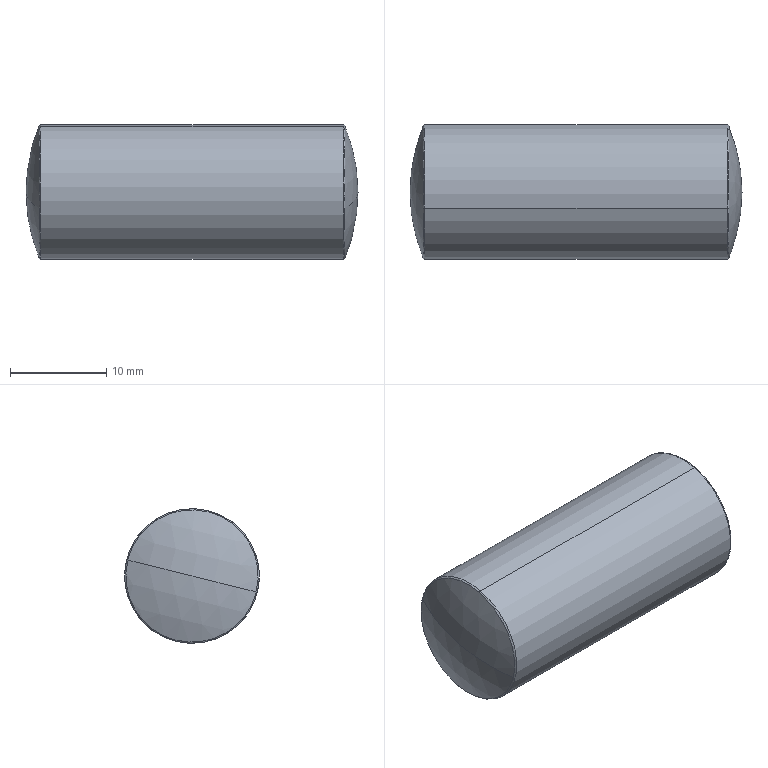Part | SolidWorks | features BaseBody 1 | 1 solid | 10 faces | box 34.5 x 14 x 14 mm | volume 5095 mm3 | torus 4 | sphere 4 | cylinder 2 | commonest cylinder face diameters 14 x2
STEP:
#1=CARTESIAN_POINT('',(58.615,29.834,6.672));
#2=VERTEX_POINT('',#1);
#3=CARTESIAN_POINT('',(58.615,38.172,1.666));
#4=VERTEX_POINT('',#3);
#5=CARTESIAN_POINT('',(58.615,31.5,0.));
#6=DIRECTION('',(-1.,0.,0.));
#7=DIRECTION('',(0.,0.2423,-0.9702));
#8=AXIS2_PLACEMENT_3D('',#5,#6,#7);
#9=CIRCLE('',#8,6.876);
#10=EDGE_CURVE('',#2,#4,#9,.T.);
#11=ORIENTED_EDGE('',*,*,#10,.F.);
#12=CARTESIAN_POINT('',(58.8,29.804,6.791));
#13=VERTEX_POINT('',#12);
#14=CARTESIAN_POINT('',(58.8,29.853,6.597));
#15=DIRECTION('',(0.,0.9702,0.2423));
#16=DIRECTION('',(0.,-0.2423,0.9702));
#17=AXIS2_PLACEMENT_3D('',#14,#15,#16);
#18=CIRCLE('',#17,0.2);
#19=EDGE_CURVE('',#2,#13,#18,.T.);
#20=ORIENTED_EDGE('',*,*,#19,.T.);
#21=CARTESIAN_POINT('',(58.8,33.196,-6.791));
#22=VERTEX_POINT('',#21);
#23=CARTESIAN_POINT('',(58.8,31.5,0.));
#24=DIRECTION('',(1.,0.,0.));
#25=DIRECTION('',(0.,0.2423,-0.9702));
#26=AXIS2_PLACEMENT_3D('',#23,#24,#25);
#27=CIRCLE('',#26,7.);
#28=EDGE_CURVE('',#22,#13,#27,.T.);
#29=ORIENTED_EDGE('',*,*,#28,.F.);
#30=CARTESIAN_POINT('',(58.615,33.166,-6.672));
#31=VERTEX_POINT('',#30);
#32=CARTESIAN_POINT('',(58.8,33.147,-6.597));
#33=DIRECTION('',(0.,-0.9702,-0.2423));
#34=DIRECTION('',(0.,0.2423,-0.9702));
#35=AXIS2_PLACEMENT_3D('',#32,#33,#34);
#36=CIRCLE('',#35,0.2);
#37=EDGE_CURVE('',#31,#22,#36,.T.);
#38=ORIENTED_EDGE('',*,*,#37,.F.);
#39=CARTESIAN_POINT('',(58.615,31.5,0.));
#40=DIRECTION('',(-1.,0.,0.));
#41=DIRECTION('',(0.,0.2423,-0.9702));
#42=AXIS2_PLACEMENT_3D('',#39,#40,#41);
#43=CIRCLE('',#42,6.876);
#44=EDGE_CURVE('',#4,#31,#43,.T.);
#45=ORIENTED_EDGE('',*,*,#44,.F.);
#46=EDGE_LOOP('',(#11,#20,#29,#38,#45));
#47=FACE_OUTER_BOUND('',#46,.T.);
#48=CARTESIAN_POINT('',(58.8,31.5,0.));
#49=DIRECTION('',(1.,0.,0.));
#50=DIRECTION('',(0.,0.2423,-0.9702));
#51=AXIS2_PLACEMENT_3D('',#48,#49,#50);
#52=TOROIDAL_SURFACE('',#51,6.8,0.2);
#53=ADVANCED_FACE('',(#47),#52,.T.);
#54=CARTESIAN_POINT('',(90.385,33.166,-6.672));
#55=VERTEX_POINT('',#54);
#56=CARTESIAN_POINT('',(90.385,38.172,1.666));
#57=VERTEX_POINT('',#56);
#58=CARTESIAN_POINT('',(90.385,31.5,0.));
#59=DIRECTION('',(1.,0.,0.));
#60=DIRECTION('',(0.,-0.2423,0.9702));
#61=AXIS2_PLACEMENT_3D('',#58,#59,#60);
#62=CIRCLE('',#61,6.876);
#63=EDGE_CURVE('',#55,#57,#62,.T.);
#64=ORIENTED_EDGE('',*,*,#63,.F.);
#65=CARTESIAN_POINT('',(90.2,33.196,-6.791));
#66=VERTEX_POINT('',#65);
#67=CARTESIAN_POINT('',(90.2,33.147,-6.597));
#68=DIRECTION('',(0.,0.9702,0.2423));
#69=DIRECTION('',(0.,-0.2423,0.9702));
#70=AXIS2_PLACEMENT_3D('',#67,#68,#69);
#71=CIRCLE('',#70,0.2);
#72=EDGE_CURVE('',#55,#66,#71,.T.);
#73=ORIENTED_EDGE('',*,*,#72,.T.);
#74=CARTESIAN_POINT('',(90.2,29.804,6.791));
#75=VERTEX_POINT('',#74);
#76=CARTESIAN_POINT('',(90.2,31.5,0.));
#77=DIRECTION('',(-1.,0.,0.));
#78=DIRECTION('',(0.,-0.2423,0.9702));
#79=AXIS2_PLACEMENT_3D('',#76,#77,#78);
#80=CIRCLE('',#79,7.);
#81=EDGE_CURVE('',#75,#66,#80,.T.);
#82=ORIENTED_EDGE('',*,*,#81,.F.);
#83=CARTESIAN_POINT('',(90.385,29.834,6.672));
#84=VERTEX_POINT('',#83);
#85=CARTESIAN_POINT('',(90.2,29.853,6.597));
#86=DIRECTION('',(0.,-0.9702,-0.2423));
#87=DIRECTION('',(0.,0.2423,-0.9702));
#88=AXIS2_PLACEMENT_3D('',#85,#86,#87);
#89=CIRCLE('',#88,0.2);
#90=EDGE_CURVE('',#84,#75,#89,.T.);
#91=ORIENTED_EDGE('',*,*,#90,.F.);
#92=CARTESIAN_POINT('',(90.385,31.5,0.));
#93=DIRECTION('',(1.,0.,0.));
#94=DIRECTION('',(0.,-0.2423,0.9702));
#95=AXIS2_PLACEMENT_3D('',#92,#93,#94);
#96=CIRCLE('',#95,6.876);
#97=EDGE_CURVE('',#57,#84,#96,.T.);
#98=ORIENTED_EDGE('',*,*,#97,.F.);
#99=EDGE_LOOP('',(#64,#73,#82,#91,#98));
#100=FACE_OUTER_BOUND('',#99,.T.);
#101=CARTESIAN_POINT('',(90.2,31.5,0.));
#102=DIRECTION('',(-1.,0.,0.));
#103=DIRECTION('',(0.,-0.2423,0.9702));
#104=AXIS2_PLACEMENT_3D('',#101,#102,#103);
#105=TOROIDAL_SURFACE('',#104,6.8,0.2);
#106=ADVANCED_FACE('',(#100),#105,.T.);
#107=ORIENTED_EDGE('',*,*,#97,.T.);
#108=CARTESIAN_POINT('',(90.385,24.828,-1.666));
#109=VERTEX_POINT('',#108);
#110=CARTESIAN_POINT('',(90.385,31.5,0.));
#111=DIRECTION('',(1.,0.,0.));
#112=DIRECTION('',(0.,-0.2423,0.9702));
#113=AXIS2_PLACEMENT_3D('',#110,#111,#112);
#114=CIRCLE('',#113,6.876);
#115=EDGE_CURVE('',#84,#109,#114,.T.);
#116=ORIENTED_EDGE('',*,*,#115,.T.);
#117=CARTESIAN_POINT('',(91.75,31.5,0.));
#118=VERTEX_POINT('',#117);
#119=CARTESIAN_POINT('',(73.75,31.5,0.));
#120=DIRECTION('',(0.,-0.2423,0.9702));
#121=DIRECTION('',(0.,-0.9702,-0.2423));
#122=AXIS2_PLACEMENT_3D('',#119,#120,#121);
#123=CIRCLE('',#122,18.);
#124=EDGE_CURVE('',#109,#118,#123,.T.);
#125=ORIENTED_EDGE('',*,*,#124,.T.);
#126=CARTESIAN_POINT('',(73.75,31.5,0.));
#127=DIRECTION('',(0.,0.2423,-0.9702));
#128=DIRECTION('',(0.,0.9702,0.2423));
#129=AXIS2_PLACEMENT_3D('',#126,#127,#128);
#130=CIRCLE('',#129,18.);
#131=EDGE_CURVE('',#57,#118,#130,.T.);
#132=ORIENTED_EDGE('',*,*,#131,.F.);
#133=EDGE_LOOP('',(#107,#116,#125,#132));
#134=FACE_OUTER_BOUND('',#133,.T.);
#135=CARTESIAN_POINT('',(73.75,31.5,0.));
#136=DIRECTION('',(0.,-0.2423,0.9702));
#137=DIRECTION('',(0.,0.9702,0.2423));
#138=AXIS2_PLACEMENT_3D('',#135,#136,#137);
#139=SPHERICAL_SURFACE('',#138,18.);
#140=ADVANCED_FACE('',(#134),#139,.T.);
#141=CARTESIAN_POINT('',(57.25,31.5,0.));
#142=VERTEX_POINT('',#141);
#143=CARTESIAN_POINT('',(58.615,24.828,-1.666));
#144=VERTEX_POINT('',#143);
#145=CARTESIAN_POINT('',(75.25,31.5,0.));
#146=DIRECTION('',(0.,-0.2423,0.9702));
#147=DIRECTION('',(0.,-0.9702,-0.2423));
#148=AXIS2_PLACEMENT_3D('',#145,#146,#147);
#149=CIRCLE('',#148,18.);
#150=EDGE_CURVE('',#142,#144,#149,.T.);
#151=ORIENTED_EDGE('',*,*,#150,.F.);
#152=CARTESIAN_POINT('',(75.25,31.5,0.));
#153=DIRECTION('',(0.,0.2423,-0.9702));
#154=DIRECTION('',(0.,0.9702,0.2423));
#155=AXIS2_PLACEMENT_3D('',#152,#153,#154);
#156=CIRCLE('',#155,18.);
#157=EDGE_CURVE('',#142,#4,#156,.T.);
#158=ORIENTED_EDGE('',*,*,#157,.T.);
#159=ORIENTED_EDGE('',*,*,#44,.T.);
#160=CARTESIAN_POINT('',(58.615,31.5,0.));
#161=DIRECTION('',(-1.,0.,0.));
#162=DIRECTION('',(0.,0.2423,-0.9702));
#163=AXIS2_PLACEMENT_3D('',#160,#161,#162);
#164=CIRCLE('',#163,6.876);
#165=EDGE_CURVE('',#31,#144,#164,.T.);
#166=ORIENTED_EDGE('',*,*,#165,.T.);
#167=EDGE_LOOP('',(#151,#158,#159,#166));
#168=FACE_OUTER_BOUND('',#167,.T.);
#169=CARTESIAN_POINT('',(75.25,31.5,0.));
#170=DIRECTION('',(0.,0.2423,-0.9702));
#171=DIRECTION('',(0.,-0.9702,-0.2423));
#172=AXIS2_PLACEMENT_3D('',#169,#170,#171);
#173=SPHERICAL_SURFACE('',#172,18.);
#174=ADVANCED_FACE('',(#168),#173,.T.);
#175=ORIENTED_EDGE('',*,*,#28,.T.);
#176=CARTESIAN_POINT('',(57.25,29.804,6.791));
#177=DIRECTION('',(1.,0.,0.));
#178=VECTOR('',#177,1000.);
#179=LINE('',#176,#178);
#180=EDGE_CURVE('',#13,#75,#179,.T.);
#181=ORIENTED_EDGE('',*,*,#180,.T.);
#182=ORIENTED_EDGE('',*,*,#81,.T.);
#183=CARTESIAN_POINT('',(57.25,33.196,-6.791));
#184=DIRECTION('',(1.,0.,0.));
#185=VECTOR('',#184,1000.);
#186=LINE('',#183,#185);
#187=EDGE_CURVE('',#22,#66,#186,.T.);
#188=ORIENTED_EDGE('',*,*,#187,.F.);
#189=EDGE_LOOP('',(#175,#181,#182,#188));
#190=FACE_OUTER_BOUND('',#189,.T.);
#191=CARTESIAN_POINT('',(57.25,31.5,0.));
#192=DIRECTION('',(1.,0.,0.));
#193=DIRECTION('',(0.,0.2423,-0.9702));
#194=AXIS2_PLACEMENT_3D('',#191,#192,#193);
#195=CYLINDRICAL_SURFACE('',#194,7.);
#196=ADVANCED_FACE('',(#190),#195,.T.);
#197=ORIENTED_EDGE('',*,*,#180,.F.);
#198=CARTESIAN_POINT('',(58.8,31.5,0.));
#199=DIRECTION('',(1.,0.,0.));
#200=DIRECTION('',(0.,0.2423,-0.9702));
#201=AXIS2_PLACEMENT_3D('',#198,#199,#200);
#202=CIRCLE('',#201,7.);
#203=EDGE_CURVE('',#13,#22,#202,.T.);
#204=ORIENTED_EDGE('',*,*,#203,.T.);
#205=ORIENTED_EDGE('',*,*,#187,.T.);
#206=CARTESIAN_POINT('',(90.2,31.5,0.));
#207=DIRECTION('',(-1.,0.,0.));
#208=DIRECTION('',(0.,-0.2423,0.9702));
#209=AXIS2_PLACEMENT_3D('',#206,#207,#208);
#210=CIRCLE('',#209,7.);
#211=EDGE_CURVE('',#66,#75,#210,.T.);
#212=ORIENTED_EDGE('',*,*,#211,.T.);
#213=EDGE_LOOP('',(#197,#204,#205,#212));
#214=FACE_OUTER_BOUND('',#213,.T.);
#215=CARTESIAN_POINT('',(57.25,31.5,0.));
#216=DIRECTION('',(1.,0.,0.));
#217=DIRECTION('',(0.,0.2423,-0.9702));
#218=AXIS2_PLACEMENT_3D('',#215,#216,#217);
#219=CYLINDRICAL_SURFACE('',#218,7.);
#220=ADVANCED_FACE('',(#214),#219,.T.);
#221=ORIENTED_EDGE('',*,*,#157,.F.);
#222=ORIENTED_EDGE('',*,*,#150,.T.);
#223=CARTESIAN_POINT('',(58.615,31.5,0.));
#224=DIRECTION('',(-1.,0.,0.));
#225=DIRECTION('',(0.,0.2423,-0.9702));
#226=AXIS2_PLACEMENT_3D('',#223,#224,#225);
#227=CIRCLE('',#226,6.876);
#228=EDGE_CURVE('',#144,#2,#227,.T.);
#229=ORIENTED_EDGE('',*,*,#228,.T.);
#230=ORIENTED_EDGE('',*,*,#10,.T.);
#231=EDGE_LOOP('',(#221,#222,#229,#230));
#232=FACE_OUTER_BOUND('',#231,.T.);
#233=CARTESIAN_POINT('',(75.25,31.5,0.));
#234=DIRECTION('',(0.,0.2423,-0.9702));
#235=DIRECTION('',(0.,-0.9702,-0.2423));
#236=AXIS2_PLACEMENT_3D('',#233,#234,#235);
#237=SPHERICAL_SURFACE('',#236,18.);
#238=ADVANCED_FACE('',(#232),#237,.T.);
#239=ORIENTED_EDGE('',*,*,#124,.F.);
#240=CARTESIAN_POINT('',(90.385,31.5,0.));
#241=DIRECTION('',(1.,0.,0.));
#242=DIRECTION('',(0.,-0.2423,0.9702));
#243=AXIS2_PLACEMENT_3D('',#240,#241,#242);
#244=CIRCLE('',#243,6.876);
#245=EDGE_CURVE('',#109,#55,#244,.T.);
#246=ORIENTED_EDGE('',*,*,#245,.T.);
#247=ORIENTED_EDGE('',*,*,#63,.T.);
#248=ORIENTED_EDGE('',*,*,#131,.T.);
#249=EDGE_LOOP('',(#239,#246,#247,#248));
#250=FACE_OUTER_BOUND('',#249,.T.);
#251=CARTESIAN_POINT('',(73.75,31.5,0.));
#252=DIRECTION('',(0.,-0.2423,0.9702));
#253=DIRECTION('',(0.,0.9702,0.2423));
#254=AXIS2_PLACEMENT_3D('',#251,#252,#253);
#255=SPHERICAL_SURFACE('',#254,18.);
#256=ADVANCED_FACE('',(#250),#255,.T.);
#257=ORIENTED_EDGE('',*,*,#72,.F.);
#258=ORIENTED_EDGE('',*,*,#245,.F.);
#259=ORIENTED_EDGE('',*,*,#115,.F.);
#260=ORIENTED_EDGE('',*,*,#90,.T.);
#261=ORIENTED_EDGE('',*,*,#211,.F.);
#262=EDGE_LOOP('',(#257,#258,#259,#260,#261));
#263=FACE_OUTER_BOUND('',#262,.T.);
#264=CARTESIAN_POINT('',(90.2,31.5,0.));
#265=DIRECTION('',(-1.,0.,0.));
#266=DIRECTION('',(0.,-0.2423,0.9702));
#267=AXIS2_PLACEMENT_3D('',#264,#265,#266);
#268=TOROIDAL_SURFACE('',#267,6.8,0.2);
#269=ADVANCED_FACE('',(#263),#268,.T.);
#270=ORIENTED_EDGE('',*,*,#19,.F.);
#271=ORIENTED_EDGE('',*,*,#228,.F.);
#272=ORIENTED_EDGE('',*,*,#165,.F.);
#273=ORIENTED_EDGE('',*,*,#37,.T.);
#274=ORIENTED_EDGE('',*,*,#203,.F.);
#275=EDGE_LOOP('',(#270,#271,#272,#273,#274));
#276=FACE_OUTER_BOUND('',#275,.T.);
#277=CARTESIAN_POINT('',(58.8,31.5,0.));
#278=DIRECTION('',(1.,0.,0.));
#279=DIRECTION('',(0.,0.2423,-0.9702));
#280=AXIS2_PLACEMENT_3D('',#277,#278,#279);
#281=TOROIDAL_SURFACE('',#280,6.8,0.2);
#282=ADVANCED_FACE('',(#276),#281,.T.);
#283=CLOSED_SHELL('',(#53,#106,#140,#174,#196,#220,#238,#256,#269,#282));
#284=MANIFOLD_SOLID_BREP('',#283);
#285=CARTESIAN_POINT('',(0.,0.,0.));
#286=DIRECTION('',(0.,0.,1.));
#287=DIRECTION('',(1.,0.,0.));
#288=AXIS2_PLACEMENT_3D('',#285,#286,#287);
#289=(LENGTH_UNIT()NAMED_UNIT(*)SI_UNIT(.MILLI.,.METRE.));
#290=UNCERTAINTY_MEASURE_WITH_UNIT(LENGTH_MEASURE(0.00001),#289,'','');
#291=(NAMED_UNIT(*)PLANE_ANGLE_UNIT()SI_UNIT($,.RADIAN.));
#292=(NAMED_UNIT(*)SI_UNIT($,.STERADIAN.)SOLID_ANGLE_UNIT());
#293=(GEOMETRIC_REPRESENTATION_CONTEXT(3)GLOBAL_UNCERTAINTY_ASSIGNED_CONTEXT((#290))GLOBAL_UNIT_ASSIGNED_CONTEXT((#289,#291,#292))REPRESENTATION_CONTEXT('',''));
#294=ADVANCED_BREP_SHAPE_REPRESENTATION('',(#284,#288),#293);